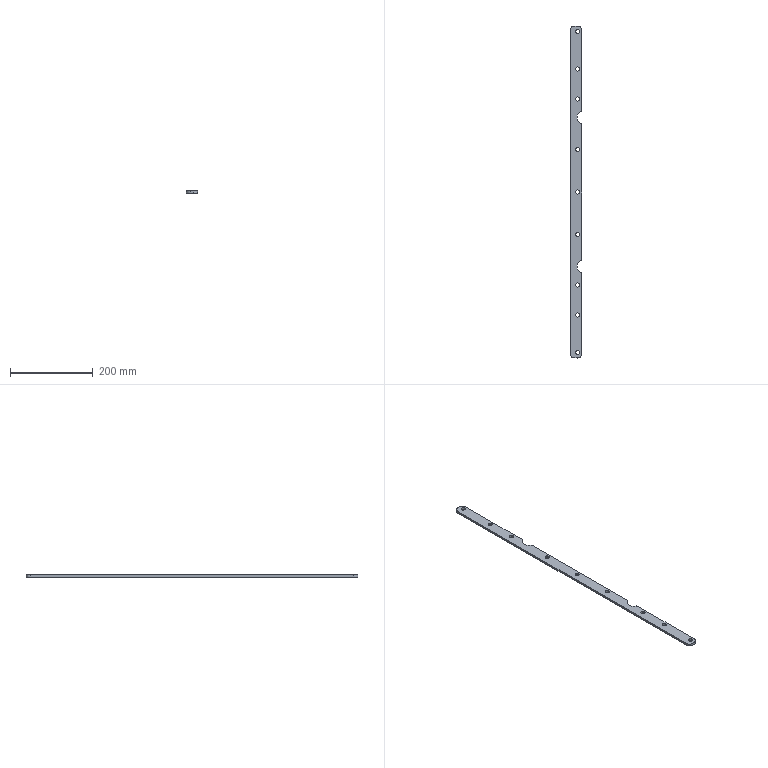Part | NX | features BREP 1 | 1 solid | 36 faces | box 27 x 803 x 5 mm | volume 101980 mm3 | cylinder 28 | plane 8 | commonest cylinder face diameters 10 x18 6 x4 20 x4 32 x2
STEP:
#1=CARTESIAN_POINT('',(541.715,-102.5,10.));
#2=VERTEX_POINT('',#1);
#3=CARTESIAN_POINT('',(551.715,-102.5,10.));
#4=VERTEX_POINT('',#3);
#5=CARTESIAN_POINT('',(546.715,-102.5,10.));
#6=DIRECTION('',(0.,0.,1.));
#7=DIRECTION('',(1.,0.,0.));
#8=AXIS2_PLACEMENT_3D('',#5,#6,#7);
#9=CIRCLE('',#8,5.);
#10=EDGE_CURVE('',#2,#4,#9,.T.);
#11=ORIENTED_EDGE('',*,*,#10,.F.);
#12=CARTESIAN_POINT('',(541.715,-102.5,15.));
#13=VERTEX_POINT('',#12);
#14=CARTESIAN_POINT('',(541.715,-102.5,20.));
#15=DIRECTION('',(0.,0.,1.));
#16=VECTOR('',#15,1000.);
#17=LINE('',#14,#16);
#18=EDGE_CURVE('',#2,#13,#17,.T.);
#19=ORIENTED_EDGE('',*,*,#18,.T.);
#20=CARTESIAN_POINT('',(551.715,-102.5,15.));
#21=VERTEX_POINT('',#20);
#22=CARTESIAN_POINT('',(546.715,-102.5,15.));
#23=DIRECTION('',(0.,0.,1.));
#24=DIRECTION('',(1.,0.,0.));
#25=AXIS2_PLACEMENT_3D('',#22,#23,#24);
#26=CIRCLE('',#25,5.);
#27=EDGE_CURVE('',#13,#21,#26,.T.);
#28=ORIENTED_EDGE('',*,*,#27,.T.);
#29=CARTESIAN_POINT('',(551.715,-102.5,20.));
#30=DIRECTION('',(0.,0.,1.));
#31=VECTOR('',#30,1000.);
#32=LINE('',#29,#31);
#33=EDGE_CURVE('',#4,#21,#32,.T.);
#34=ORIENTED_EDGE('',*,*,#33,.F.);
#35=EDGE_LOOP('',(#11,#19,#28,#34));
#36=FACE_BOUND('',#35,.T.);
#37=CARTESIAN_POINT('',(546.715,-102.5,20.));
#38=DIRECTION('',(0.,0.,1.));
#39=DIRECTION('',(-1.,0.,0.));
#40=AXIS2_PLACEMENT_3D('',#37,#38,#39);
#41=CYLINDRICAL_SURFACE('',#40,5.);
#42=ADVANCED_FACE('',(#36),#41,.F.);
#43=CARTESIAN_POINT('',(541.715,-0.0003019,10.));
#44=VERTEX_POINT('',#43);
#45=CARTESIAN_POINT('',(551.715,-0.0003019,10.));
#46=VERTEX_POINT('',#45);
#47=CARTESIAN_POINT('',(546.715,-0.0003019,10.));
#48=DIRECTION('',(0.,0.,1.));
#49=DIRECTION('',(1.,0.,0.));
#50=AXIS2_PLACEMENT_3D('',#47,#48,#49);
#51=CIRCLE('',#50,5.);
#52=EDGE_CURVE('',#44,#46,#51,.T.);
#53=ORIENTED_EDGE('',*,*,#52,.F.);
#54=CARTESIAN_POINT('',(541.715,-0.0003019,15.));
#55=VERTEX_POINT('',#54);
#56=CARTESIAN_POINT('',(541.715,-0.0003019,20.));
#57=DIRECTION('',(0.,0.,1.));
#58=VECTOR('',#57,1000.);
#59=LINE('',#56,#58);
#60=EDGE_CURVE('',#44,#55,#59,.T.);
#61=ORIENTED_EDGE('',*,*,#60,.T.);
#62=CARTESIAN_POINT('',(551.715,-0.0003019,15.));
#63=VERTEX_POINT('',#62);
#64=CARTESIAN_POINT('',(546.715,-0.0003019,15.));
#65=DIRECTION('',(0.,0.,1.));
#66=DIRECTION('',(1.,0.,0.));
#67=AXIS2_PLACEMENT_3D('',#64,#65,#66);
#68=CIRCLE('',#67,5.);
#69=EDGE_CURVE('',#55,#63,#68,.T.);
#70=ORIENTED_EDGE('',*,*,#69,.T.);
#71=CARTESIAN_POINT('',(551.715,-0.0003019,20.));
#72=DIRECTION('',(0.,0.,1.));
#73=VECTOR('',#72,1000.);
#74=LINE('',#71,#73);
#75=EDGE_CURVE('',#46,#63,#74,.T.);
#76=ORIENTED_EDGE('',*,*,#75,.F.);
#77=EDGE_LOOP('',(#53,#61,#70,#76));
#78=FACE_BOUND('',#77,.T.);
#79=CARTESIAN_POINT('',(546.715,-0.0003019,20.));
#80=DIRECTION('',(0.,0.,1.));
#81=DIRECTION('',(-1.,0.,0.));
#82=AXIS2_PLACEMENT_3D('',#79,#80,#81);
#83=CYLINDRICAL_SURFACE('',#82,5.);
#84=ADVANCED_FACE('',(#78),#83,.F.);
#85=CARTESIAN_POINT('',(541.715,102.5,10.));
#86=VERTEX_POINT('',#85);
#87=CARTESIAN_POINT('',(551.715,102.5,10.));
#88=VERTEX_POINT('',#87);
#89=CARTESIAN_POINT('',(546.715,102.5,10.));
#90=DIRECTION('',(0.,0.,1.));
#91=DIRECTION('',(1.,0.,0.));
#92=AXIS2_PLACEMENT_3D('',#89,#90,#91);
#93=CIRCLE('',#92,5.);
#94=EDGE_CURVE('',#86,#88,#93,.T.);
#95=ORIENTED_EDGE('',*,*,#94,.F.);
#96=CARTESIAN_POINT('',(541.715,102.5,15.));
#97=VERTEX_POINT('',#96);
#98=CARTESIAN_POINT('',(541.715,102.5,20.));
#99=DIRECTION('',(0.,0.,1.));
#100=VECTOR('',#99,1000.);
#101=LINE('',#98,#100);
#102=EDGE_CURVE('',#86,#97,#101,.T.);
#103=ORIENTED_EDGE('',*,*,#102,.T.);
#104=CARTESIAN_POINT('',(551.715,102.5,15.));
#105=VERTEX_POINT('',#104);
#106=CARTESIAN_POINT('',(546.715,102.5,15.));
#107=DIRECTION('',(0.,0.,1.));
#108=DIRECTION('',(1.,0.,0.));
#109=AXIS2_PLACEMENT_3D('',#106,#107,#108);
#110=CIRCLE('',#109,5.);
#111=EDGE_CURVE('',#97,#105,#110,.T.);
#112=ORIENTED_EDGE('',*,*,#111,.T.);
#113=CARTESIAN_POINT('',(551.715,102.5,20.));
#114=DIRECTION('',(0.,0.,1.));
#115=VECTOR('',#114,1000.);
#116=LINE('',#113,#115);
#117=EDGE_CURVE('',#88,#105,#116,.T.);
#118=ORIENTED_EDGE('',*,*,#117,.F.);
#119=EDGE_LOOP('',(#95,#103,#112,#118));
#120=FACE_BOUND('',#119,.T.);
#121=CARTESIAN_POINT('',(546.715,102.5,20.));
#122=DIRECTION('',(0.,0.,1.));
#123=DIRECTION('',(-1.,0.,0.));
#124=AXIS2_PLACEMENT_3D('',#121,#122,#123);
#125=CYLINDRICAL_SURFACE('',#124,5.);
#126=ADVANCED_FACE('',(#120),#125,.F.);
#127=CARTESIAN_POINT('',(541.715,225.,10.));
#128=VERTEX_POINT('',#127);
#129=CARTESIAN_POINT('',(551.715,225.,10.));
#130=VERTEX_POINT('',#129);
#131=CARTESIAN_POINT('',(546.715,225.,10.));
#132=DIRECTION('',(0.,0.,1.));
#133=DIRECTION('',(1.,0.,0.));
#134=AXIS2_PLACEMENT_3D('',#131,#132,#133);
#135=CIRCLE('',#134,5.);
#136=EDGE_CURVE('',#128,#130,#135,.T.);
#137=ORIENTED_EDGE('',*,*,#136,.F.);
#138=CARTESIAN_POINT('',(541.715,225.,15.));
#139=VERTEX_POINT('',#138);
#140=CARTESIAN_POINT('',(541.715,225.,20.));
#141=DIRECTION('',(0.,0.,1.));
#142=VECTOR('',#141,1000.);
#143=LINE('',#140,#142);
#144=EDGE_CURVE('',#128,#139,#143,.T.);
#145=ORIENTED_EDGE('',*,*,#144,.T.);
#146=CARTESIAN_POINT('',(551.715,225.,15.));
#147=VERTEX_POINT('',#146);
#148=CARTESIAN_POINT('',(546.715,225.,15.));
#149=DIRECTION('',(0.,0.,1.));
#150=DIRECTION('',(1.,0.,0.));
#151=AXIS2_PLACEMENT_3D('',#148,#149,#150);
#152=CIRCLE('',#151,5.);
#153=EDGE_CURVE('',#139,#147,#152,.T.);
#154=ORIENTED_EDGE('',*,*,#153,.T.);
#155=CARTESIAN_POINT('',(551.715,225.,20.));
#156=DIRECTION('',(0.,0.,1.));
#157=VECTOR('',#156,1000.);
#158=LINE('',#155,#157);
#159=EDGE_CURVE('',#130,#147,#158,.T.);
#160=ORIENTED_EDGE('',*,*,#159,.F.);
#161=EDGE_LOOP('',(#137,#145,#154,#160));
#162=FACE_BOUND('',#161,.T.);
#163=CARTESIAN_POINT('',(546.715,225.,20.));
#164=DIRECTION('',(0.,0.,1.));
#165=DIRECTION('',(-1.,0.,0.));
#166=AXIS2_PLACEMENT_3D('',#163,#164,#165);
#167=CYLINDRICAL_SURFACE('',#166,5.);
#168=ADVANCED_FACE('',(#162),#167,.F.);
#169=CARTESIAN_POINT('',(541.715,297.5,10.));
#170=VERTEX_POINT('',#169);
#171=CARTESIAN_POINT('',(551.715,297.5,10.));
#172=VERTEX_POINT('',#171);
#173=CARTESIAN_POINT('',(546.715,297.5,10.));
#174=DIRECTION('',(0.,0.,1.));
#175=DIRECTION('',(1.,0.,0.));
#176=AXIS2_PLACEMENT_3D('',#173,#174,#175);
#177=CIRCLE('',#176,5.);
#178=EDGE_CURVE('',#170,#172,#177,.T.);
#179=ORIENTED_EDGE('',*,*,#178,.F.);
#180=CARTESIAN_POINT('',(541.715,297.5,15.));
#181=VERTEX_POINT('',#180);
#182=CARTESIAN_POINT('',(541.715,297.5,20.));
#183=DIRECTION('',(0.,0.,1.));
#184=VECTOR('',#183,1000.);
#185=LINE('',#182,#184);
#186=EDGE_CURVE('',#170,#181,#185,.T.);
#187=ORIENTED_EDGE('',*,*,#186,.T.);
#188=CARTESIAN_POINT('',(551.715,297.5,15.));
#189=VERTEX_POINT('',#188);
#190=CARTESIAN_POINT('',(546.715,297.5,15.));
#191=DIRECTION('',(0.,0.,1.));
#192=DIRECTION('',(1.,0.,0.));
#193=AXIS2_PLACEMENT_3D('',#190,#191,#192);
#194=CIRCLE('',#193,5.);
#195=EDGE_CURVE('',#181,#189,#194,.T.);
#196=ORIENTED_EDGE('',*,*,#195,.T.);
#197=CARTESIAN_POINT('',(551.715,297.5,20.));
#198=DIRECTION('',(0.,0.,1.));
#199=VECTOR('',#198,1000.);
#200=LINE('',#197,#199);
#201=EDGE_CURVE('',#172,#189,#200,.T.);
#202=ORIENTED_EDGE('',*,*,#201,.F.);
#203=EDGE_LOOP('',(#179,#187,#196,#202));
#204=FACE_BOUND('',#203,.T.);
#205=CARTESIAN_POINT('',(546.715,297.5,20.));
#206=DIRECTION('',(0.,0.,1.));
#207=DIRECTION('',(-1.,0.,0.));
#208=AXIS2_PLACEMENT_3D('',#205,#206,#207);
#209=CYLINDRICAL_SURFACE('',#208,5.);
#210=ADVANCED_FACE('',(#204),#209,.F.);
#211=CARTESIAN_POINT('',(541.715,-297.5,10.));
#212=VERTEX_POINT('',#211);
#213=CARTESIAN_POINT('',(551.715,-297.5,10.));
#214=VERTEX_POINT('',#213);
#215=CARTESIAN_POINT('',(546.715,-297.5,10.));
#216=DIRECTION('',(0.,0.,1.));
#217=DIRECTION('',(1.,0.,0.));
#218=AXIS2_PLACEMENT_3D('',#215,#216,#217);
#219=CIRCLE('',#218,5.);
#220=EDGE_CURVE('',#212,#214,#219,.T.);
#221=ORIENTED_EDGE('',*,*,#220,.F.);
#222=CARTESIAN_POINT('',(541.715,-297.5,15.));
#223=VERTEX_POINT('',#222);
#224=CARTESIAN_POINT('',(541.715,-297.5,20.));
#225=DIRECTION('',(0.,0.,1.));
#226=VECTOR('',#225,1000.);
#227=LINE('',#224,#226);
#228=EDGE_CURVE('',#212,#223,#227,.T.);
#229=ORIENTED_EDGE('',*,*,#228,.T.);
#230=CARTESIAN_POINT('',(551.715,-297.5,15.));
#231=VERTEX_POINT('',#230);
#232=CARTESIAN_POINT('',(546.715,-297.5,15.));
#233=DIRECTION('',(0.,0.,1.));
#234=DIRECTION('',(1.,0.,0.));
#235=AXIS2_PLACEMENT_3D('',#232,#233,#234);
#236=CIRCLE('',#235,5.);
#237=EDGE_CURVE('',#223,#231,#236,.T.);
#238=ORIENTED_EDGE('',*,*,#237,.T.);
#239=CARTESIAN_POINT('',(551.715,-297.5,20.));
#240=DIRECTION('',(0.,0.,1.));
#241=VECTOR('',#240,1000.);
#242=LINE('',#239,#241);
#243=EDGE_CURVE('',#214,#231,#242,.T.);
#244=ORIENTED_EDGE('',*,*,#243,.F.);
#245=EDGE_LOOP('',(#221,#229,#238,#244));
#246=FACE_BOUND('',#245,.T.);
#247=CARTESIAN_POINT('',(546.715,-297.5,20.));
#248=DIRECTION('',(0.,0.,1.));
#249=DIRECTION('',(-1.,0.,0.));
#250=AXIS2_PLACEMENT_3D('',#247,#248,#249);
#251=CYLINDRICAL_SURFACE('',#250,5.);
#252=ADVANCED_FACE('',(#246),#251,.F.);
#253=CARTESIAN_POINT('',(541.715,-388.5,10.));
#254=VERTEX_POINT('',#253);
#255=CARTESIAN_POINT('',(551.715,-388.5,10.));
#256=VERTEX_POINT('',#255);
#257=CARTESIAN_POINT('',(546.715,-388.5,10.));
#258=DIRECTION('',(0.,0.,1.));
#259=DIRECTION('',(1.,0.,0.));
#260=AXIS2_PLACEMENT_3D('',#257,#258,#259);
#261=CIRCLE('',#260,5.);
#262=EDGE_CURVE('',#254,#256,#261,.T.);
#263=ORIENTED_EDGE('',*,*,#262,.F.);
#264=CARTESIAN_POINT('',(541.715,-388.5,15.));
#265=VERTEX_POINT('',#264);
#266=CARTESIAN_POINT('',(541.715,-388.5,15.));
#267=DIRECTION('',(0.,0.,1.));
#268=VECTOR('',#267,1000.);
#269=LINE('',#266,#268);
#270=EDGE_CURVE('',#254,#265,#269,.T.);
#271=ORIENTED_EDGE('',*,*,#270,.T.);
#272=CARTESIAN_POINT('',(551.715,-388.5,15.));
#273=VERTEX_POINT('',#272);
#274=CARTESIAN_POINT('',(546.715,-388.5,15.));
#275=DIRECTION('',(0.,0.,1.));
#276=DIRECTION('',(1.,0.,0.));
#277=AXIS2_PLACEMENT_3D('',#274,#275,#276);
#278=CIRCLE('',#277,5.);
#279=EDGE_CURVE('',#265,#273,#278,.T.);
#280=ORIENTED_EDGE('',*,*,#279,.T.);
#281=CARTESIAN_POINT('',(551.715,-388.5,15.));
#282=DIRECTION('',(0.,0.,1.));
#283=VECTOR('',#282,1000.);
#284=LINE('',#281,#283);
#285=EDGE_CURVE('',#256,#273,#284,.T.);
#286=ORIENTED_EDGE('',*,*,#285,.F.);
#287=EDGE_LOOP('',(#263,#271,#280,#286));
#288=FACE_BOUND('',#287,.T.);
#289=CARTESIAN_POINT('',(546.715,-388.5,15.));
#290=DIRECTION('',(0.,0.,1.));
#291=DIRECTION('',(-1.,0.,0.));
#292=AXIS2_PLACEMENT_3D('',#289,#290,#291);
#293=CYLINDRICAL_SURFACE('',#292,5.);
#294=ADVANCED_FACE('',(#288),#293,.F.);
#295=CARTESIAN_POINT('',(541.715,388.5,10.));
#296=VERTEX_POINT('',#295);
#297=CARTESIAN_POINT('',(551.715,388.5,10.));
#298=VERTEX_POINT('',#297);
#299=CARTESIAN_POINT('',(546.715,388.5,10.));
#300=DIRECTION('',(0.,0.,1.));
#301=DIRECTION('',(1.,0.,0.));
#302=AXIS2_PLACEMENT_3D('',#299,#300,#301);
#303=CIRCLE('',#302,5.);
#304=EDGE_CURVE('',#296,#298,#303,.T.);
#305=ORIENTED_EDGE('',*,*,#304,.F.);
#306=CARTESIAN_POINT('',(541.715,388.5,15.));
#307=VERTEX_POINT('',#306);
#308=CARTESIAN_POINT('',(541.715,388.5,15.));
#309=DIRECTION('',(0.,0.,1.));
#310=VECTOR('',#309,1000.);
#311=LINE('',#308,#310);
#312=EDGE_CURVE('',#296,#307,#311,.T.);
#313=ORIENTED_EDGE('',*,*,#312,.T.);
#314=CARTESIAN_POINT('',(551.715,388.5,15.));
#315=VERTEX_POINT('',#314);
#316=CARTESIAN_POINT('',(546.715,388.5,15.));
#317=DIRECTION('',(0.,0.,1.));
#318=DIRECTION('',(1.,0.,0.));
#319=AXIS2_PLACEMENT_3D('',#316,#317,#318);
#320=CIRCLE('',#319,5.);
#321=EDGE_CURVE('',#307,#315,#320,.T.);
#322=ORIENTED_EDGE('',*,*,#321,.T.);
#323=CARTESIAN_POINT('',(551.715,388.5,15.));
#324=DIRECTION('',(0.,0.,1.));
#325=VECTOR('',#324,1000.);
#326=LINE('',#323,#325);
#327=EDGE_CURVE('',#298,#315,#326,.T.);
#328=ORIENTED_EDGE('',*,*,#327,.F.);
#329=EDGE_LOOP('',(#305,#313,#322,#328));
#330=FACE_BOUND('',#329,.T.);
#331=CARTESIAN_POINT('',(546.715,388.5,15.));
#332=DIRECTION('',(0.,0.,1.));
#333=DIRECTION('',(-1.,0.,0.));
#334=AXIS2_PLACEMENT_3D('',#331,#332,#333);
#335=CYLINDRICAL_SURFACE('',#334,5.);
#336=ADVANCED_FACE('',(#330),#335,.F.);
#337=CARTESIAN_POINT('',(541.715,-225.,10.));
#338=VERTEX_POINT('',#337);
#339=CARTESIAN_POINT('',(551.715,-225.,10.));
#340=VERTEX_POINT('',#339);
#341=CARTESIAN_POINT('',(546.715,-225.,10.));
#342=DIRECTION('',(0.,0.,1.));
#343=DIRECTION('',(1.,0.,0.));
#344=AXIS2_PLACEMENT_3D('',#341,#342,#343);
#345=CIRCLE('',#344,5.);
#346=EDGE_CURVE('',#338,#340,#345,.T.);
#347=ORIENTED_EDGE('',*,*,#346,.F.);
#348=CARTESIAN_POINT('',(541.715,-225.,15.));
#349=VERTEX_POINT('',#348);
#350=CARTESIAN_POINT('',(541.715,-225.,20.));
#351=DIRECTION('',(0.,0.,1.));
#352=VECTOR('',#351,1000.);
#353=LINE('',#350,#352);
#354=EDGE_CURVE('',#338,#349,#353,.T.);
#355=ORIENTED_EDGE('',*,*,#354,.T.);
#356=CARTESIAN_POINT('',(551.715,-225.,15.));
#357=VERTEX_POINT('',#356);
#358=CARTESIAN_POINT('',(546.715,-225.,15.));
#359=DIRECTION('',(0.,0.,1.));
#360=DIRECTION('',(1.,0.,0.));
#361=AXIS2_PLACEMENT_3D('',#358,#359,#360);
#362=CIRCLE('',#361,5.);
#363=EDGE_CURVE('',#349,#357,#362,.T.);
#364=ORIENTED_EDGE('',*,*,#363,.T.);
#365=CARTESIAN_POINT('',(551.715,-225.,20.));
#366=DIRECTION('',(0.,0.,1.));
#367=VECTOR('',#366,1000.);
#368=LINE('',#365,#367);
#369=EDGE_CURVE('',#340,#357,#368,.T.);
#370=ORIENTED_EDGE('',*,*,#369,.F.);
#371=EDGE_LOOP('',(#347,#355,#364,#370));
#372=FACE_BOUND('',#371,.T.);
#373=CARTESIAN_POINT('',(546.715,-225.,20.));
#374=DIRECTION('',(0.,0.,1.));
#375=DIRECTION('',(-1.,0.,0.));
#376=AXIS2_PLACEMENT_3D('',#373,#374,#375);
#377=CYLINDRICAL_SURFACE('',#376,5.);
#378=ADVANCED_FACE('',(#372),#377,.F.);
#379=CARTESIAN_POINT('',(556.16,-197.334,15.));
#380=VERTEX_POINT('',#379);
#381=CARTESIAN_POINT('',(556.16,-391.5,15.));
#382=VERTEX_POINT('',#381);
#383=CARTESIAN_POINT('',(556.16,-0.0003019,15.));
#384=DIRECTION('',(0.,-1.,0.));
#385=VECTOR('',#384,1000.);
#386=LINE('',#383,#385);
#387=EDGE_CURVE('',#380,#382,#386,.T.);
#388=ORIENTED_EDGE('',*,*,#387,.F.);
#389=CARTESIAN_POINT('',(554.423,-194.613,15.));
#390=VERTEX_POINT('',#389);
#391=CARTESIAN_POINT('',(553.16,-197.334,15.));
#392=DIRECTION('',(0.,0.,-1.));
#393=DIRECTION('',(-1.,0.,0.));
#394=AXIS2_PLACEMENT_3D('',#391,#392,#393);
#395=CIRCLE('',#394,3.);
#396=EDGE_CURVE('',#390,#380,#395,.T.);
#397=ORIENTED_EDGE('',*,*,#396,.F.);
#398=CARTESIAN_POINT('',(554.423,-165.587,15.));
#399=VERTEX_POINT('',#398);
#400=CARTESIAN_POINT('',(561.16,-180.1,15.));
#401=DIRECTION('',(0.,0.,1.));
#402=DIRECTION('',(1.,0.,0.));
#403=AXIS2_PLACEMENT_3D('',#400,#401,#402);
#404=CIRCLE('',#403,16.);
#405=EDGE_CURVE('',#399,#390,#404,.T.);
#406=ORIENTED_EDGE('',*,*,#405,.F.);
#407=CARTESIAN_POINT('',(556.16,-162.866,15.));
#408=VERTEX_POINT('',#407);
#409=CARTESIAN_POINT('',(553.16,-162.866,15.));
#410=DIRECTION('',(0.,0.,-1.));
#411=DIRECTION('',(1.,0.,0.));
#412=AXIS2_PLACEMENT_3D('',#409,#410,#411);
#413=CIRCLE('',#412,3.);
#414=EDGE_CURVE('',#408,#399,#413,.T.);
#415=ORIENTED_EDGE('',*,*,#414,.F.);
#416=CARTESIAN_POINT('',(556.16,162.866,15.));
#417=VERTEX_POINT('',#416);
#418=CARTESIAN_POINT('',(556.16,-0.0003019,15.));
#419=DIRECTION('',(0.,-1.,0.));
#420=VECTOR('',#419,1000.);
#421=LINE('',#418,#420);
#422=EDGE_CURVE('',#417,#408,#421,.T.);
#423=ORIENTED_EDGE('',*,*,#422,.F.);
#424=CARTESIAN_POINT('',(554.423,165.587,15.));
#425=VERTEX_POINT('',#424);
#426=CARTESIAN_POINT('',(553.16,162.866,15.));
#427=DIRECTION('',(0.,0.,-1.));
#428=DIRECTION('',(-1.,0.,0.));
#429=AXIS2_PLACEMENT_3D('',#426,#427,#428);
#430=CIRCLE('',#429,3.);
#431=EDGE_CURVE('',#425,#417,#430,.T.);
#432=ORIENTED_EDGE('',*,*,#431,.F.);
#433=CARTESIAN_POINT('',(554.423,194.613,15.));
#434=VERTEX_POINT('',#433);
#435=CARTESIAN_POINT('',(561.16,180.1,15.));
#436=DIRECTION('',(0.,0.,1.));
#437=DIRECTION('',(1.,0.,0.));
#438=AXIS2_PLACEMENT_3D('',#435,#436,#437);
#439=CIRCLE('',#438,16.);
#440=EDGE_CURVE('',#434,#425,#439,.T.);
#441=ORIENTED_EDGE('',*,*,#440,.F.);
#442=CARTESIAN_POINT('',(556.16,197.334,15.));
#443=VERTEX_POINT('',#442);
#444=CARTESIAN_POINT('',(553.16,197.334,15.));
#445=DIRECTION('',(0.,0.,-1.));
#446=DIRECTION('',(1.,0.,0.));
#447=AXIS2_PLACEMENT_3D('',#444,#445,#446);
#448=CIRCLE('',#447,3.);
#449=EDGE_CURVE('',#443,#434,#448,.T.);
#450=ORIENTED_EDGE('',*,*,#449,.F.);
#451=CARTESIAN_POINT('',(556.16,391.5,15.));
#452=VERTEX_POINT('',#451);
#453=CARTESIAN_POINT('',(556.16,-0.0003019,15.));
#454=DIRECTION('',(0.,-1.,0.));
#455=VECTOR('',#454,1000.);
#456=LINE('',#453,#455);
#457=EDGE_CURVE('',#452,#443,#456,.T.);
#458=ORIENTED_EDGE('',*,*,#457,.F.);
#459=CARTESIAN_POINT('',(546.16,401.5,15.));
#460=VERTEX_POINT('',#459);
#461=CARTESIAN_POINT('',(546.16,391.5,15.));
#462=DIRECTION('',(0.,0.,-1.));
#463=DIRECTION('',(1.,0.,0.));
#464=AXIS2_PLACEMENT_3D('',#461,#462,#463);
#465=CIRCLE('',#464,10.);
#466=EDGE_CURVE('',#460,#452,#465,.T.);
#467=ORIENTED_EDGE('',*,*,#466,.F.);
#468=CARTESIAN_POINT('',(539.16,401.5,15.));
#469=VERTEX_POINT('',#468);
#470=CARTESIAN_POINT('',(-11.34,401.5,15.));
#471=DIRECTION('',(1.,0.,0.));
#472=VECTOR('',#471,1000.);
#473=LINE('',#470,#472);
#474=EDGE_CURVE('',#469,#460,#473,.T.);
#475=ORIENTED_EDGE('',*,*,#474,.F.);
#476=CARTESIAN_POINT('',(529.16,391.5,15.));
#477=VERTEX_POINT('',#476);
#478=CARTESIAN_POINT('',(539.16,391.5,15.));
#479=DIRECTION('',(0.,0.,-1.));
#480=DIRECTION('',(-1.,0.,0.));
#481=AXIS2_PLACEMENT_3D('',#478,#479,#480);
#482=CIRCLE('',#481,10.);
#483=EDGE_CURVE('',#477,#469,#482,.T.);
#484=ORIENTED_EDGE('',*,*,#483,.F.);
#485=CARTESIAN_POINT('',(529.16,-391.5,15.));
#486=VERTEX_POINT('',#485);
#487=CARTESIAN_POINT('',(529.16,-0.0003019,15.));
#488=DIRECTION('',(0.,1.,0.));
#489=VECTOR('',#488,1000.);
#490=LINE('',#487,#489);
#491=EDGE_CURVE('',#486,#477,#490,.T.);
#492=ORIENTED_EDGE('',*,*,#491,.F.);
#493=CARTESIAN_POINT('',(539.16,-401.5,15.));
#494=VERTEX_POINT('',#493);
#495=CARTESIAN_POINT('',(539.16,-391.5,15.));
#496=DIRECTION('',(0.,0.,-1.));
#497=DIRECTION('',(-1.,0.,0.));
#498=AXIS2_PLACEMENT_3D('',#495,#496,#497);
#499=CIRCLE('',#498,10.);
#500=EDGE_CURVE('',#494,#486,#499,.T.);
#501=ORIENTED_EDGE('',*,*,#500,.F.);
#502=CARTESIAN_POINT('',(546.16,-401.5,15.));
#503=VERTEX_POINT('',#502);
#504=CARTESIAN_POINT('',(-11.34,-401.5,15.));
#505=DIRECTION('',(-1.,0.,0.));
#506=VECTOR('',#505,1000.);
#507=LINE('',#504,#506);
#508=EDGE_CURVE('',#503,#494,#507,.T.);
#509=ORIENTED_EDGE('',*,*,#508,.F.);
#510=CARTESIAN_POINT('',(546.16,-391.5,15.));
#511=DIRECTION('',(0.,0.,-1.));
#512=DIRECTION('',(1.,0.,0.));
#513=AXIS2_PLACEMENT_3D('',#510,#511,#512);
#514=CIRCLE('',#513,10.);
#515=EDGE_CURVE('',#382,#503,#514,.T.);
#516=ORIENTED_EDGE('',*,*,#515,.F.);
#517=EDGE_LOOP('',(#388,#397,#406,#415,#423,#432,#441,#450,#458,#467,#475,#484,#492,#501,#509,#516));
#518=FACE_BOUND('',#517,.T.);
#519=CARTESIAN_POINT('',(546.715,-102.5,15.));
#520=DIRECTION('',(0.,0.,1.));
#521=DIRECTION('',(1.,0.,0.));
#522=AXIS2_PLACEMENT_3D('',#519,#520,#521);
#523=CIRCLE('',#522,5.);
#524=EDGE_CURVE('',#21,#13,#523,.T.);
#525=ORIENTED_EDGE('',*,*,#524,.F.);
#526=ORIENTED_EDGE('',*,*,#27,.F.);
#527=EDGE_LOOP('',(#525,#526));
#528=FACE_BOUND('',#527,.T.);
#529=CARTESIAN_POINT('',(546.715,-0.0003019,15.));
#530=DIRECTION('',(0.,0.,1.));
#531=DIRECTION('',(1.,0.,0.));
#532=AXIS2_PLACEMENT_3D('',#529,#530,#531);
#533=CIRCLE('',#532,5.);
#534=EDGE_CURVE('',#63,#55,#533,.T.);
#535=ORIENTED_EDGE('',*,*,#534,.F.);
#536=ORIENTED_EDGE('',*,*,#69,.F.);
#537=EDGE_LOOP('',(#535,#536));
#538=FACE_BOUND('',#537,.T.);
#539=CARTESIAN_POINT('',(546.715,102.5,15.));
#540=DIRECTION('',(0.,0.,1.));
#541=DIRECTION('',(1.,0.,0.));
#542=AXIS2_PLACEMENT_3D('',#539,#540,#541);
#543=CIRCLE('',#542,5.);
#544=EDGE_CURVE('',#105,#97,#543,.T.);
#545=ORIENTED_EDGE('',*,*,#544,.F.);
#546=ORIENTED_EDGE('',*,*,#111,.F.);
#547=EDGE_LOOP('',(#545,#546));
#548=FACE_BOUND('',#547,.T.);
#549=CARTESIAN_POINT('',(546.715,225.,15.));
#550=DIRECTION('',(0.,0.,1.));
#551=DIRECTION('',(1.,0.,0.));
#552=AXIS2_PLACEMENT_3D('',#549,#550,#551);
#553=CIRCLE('',#552,5.);
#554=EDGE_CURVE('',#147,#139,#553,.T.);
#555=ORIENTED_EDGE('',*,*,#554,.F.);
#556=ORIENTED_EDGE('',*,*,#153,.F.);
#557=EDGE_LOOP('',(#555,#556));
#558=FACE_BOUND('',#557,.T.);
#559=CARTESIAN_POINT('',(546.715,297.5,15.));
#560=DIRECTION('',(0.,0.,1.));
#561=DIRECTION('',(1.,0.,0.));
#562=AXIS2_PLACEMENT_3D('',#559,#560,#561);
#563=CIRCLE('',#562,5.);
#564=EDGE_CURVE('',#189,#181,#563,.T.);
#565=ORIENTED_EDGE('',*,*,#564,.F.);
#566=ORIENTED_EDGE('',*,*,#195,.F.);
#567=EDGE_LOOP('',(#565,#566));
#568=FACE_BOUND('',#567,.T.);
#569=CARTESIAN_POINT('',(546.715,-297.5,15.));
#570=DIRECTION('',(0.,0.,1.));
#571=DIRECTION('',(1.,0.,0.));
#572=AXIS2_PLACEMENT_3D('',#569,#570,#571);
#573=CIRCLE('',#572,5.);
#574=EDGE_CURVE('',#231,#223,#573,.T.);
#575=ORIENTED_EDGE('',*,*,#574,.F.);
#576=ORIENTED_EDGE('',*,*,#237,.F.);
#577=EDGE_LOOP('',(#575,#576));
#578=FACE_BOUND('',#577,.T.);
#579=CARTESIAN_POINT('',(546.715,-388.5,15.));
#580=DIRECTION('',(0.,0.,1.));
#581=DIRECTION('',(1.,0.,0.));
#582=AXIS2_PLACEMENT_3D('',#579,#580,#581);
#583=CIRCLE('',#582,5.);
#584=EDGE_CURVE('',#273,#265,#583,.T.);
#585=ORIENTED_EDGE('',*,*,#584,.F.);
#586=ORIENTED_EDGE('',*,*,#279,.F.);
#587=EDGE_LOOP('',(#585,#586));
#588=FACE_BOUND('',#587,.T.);
#589=CARTESIAN_POINT('',(546.715,388.5,15.));
#590=DIRECTION('',(0.,0.,1.));
#591=DIRECTION('',(1.,0.,0.));
#592=AXIS2_PLACEMENT_3D('',#589,#590,#591);
#593=CIRCLE('',#592,5.);
#594=EDGE_CURVE('',#315,#307,#593,.T.);
#595=ORIENTED_EDGE('',*,*,#594,.F.);
#596=ORIENTED_EDGE('',*,*,#321,.F.);
#597=EDGE_LOOP('',(#595,#596));
#598=FACE_BOUND('',#597,.T.);
#599=CARTESIAN_POINT('',(546.715,-225.,15.));
#600=DIRECTION('',(0.,0.,1.));
#601=DIRECTION('',(1.,0.,0.));
#602=AXIS2_PLACEMENT_3D('',#599,#600,#601);
#603=CIRCLE('',#602,5.);
#604=EDGE_CURVE('',#357,#349,#603,.T.);
#605=ORIENTED_EDGE('',*,*,#604,.F.);
#606=ORIENTED_EDGE('',*,*,#363,.F.);
#607=EDGE_LOOP('',(#605,#606));
#608=FACE_BOUND('',#607,.T.);
#609=CARTESIAN_POINT('',(-11.34,-0.0003019,15.));
#610=DIRECTION('',(0.,0.,-1.));
#611=DIRECTION('',(1.,0.,0.));
#612=AXIS2_PLACEMENT_3D('',#609,#610,#611);
#613=PLANE('',#612);
#614=ADVANCED_FACE('',(#518,#528,#538,#548,#558,#568,#578,#588,#598,#608),#613,.F.);
#615=CARTESIAN_POINT('',(556.16,-391.5,10.));
#616=VERTEX_POINT('',#615);
#617=CARTESIAN_POINT('',(556.16,-391.5,-2.53));
#618=DIRECTION('',(0.,0.,1.));
#619=VECTOR('',#618,1000.);
#620=LINE('',#617,#619);
#621=EDGE_CURVE('',#616,#382,#620,.T.);
#622=ORIENTED_EDGE('',*,*,#621,.T.);
#623=ORIENTED_EDGE('',*,*,#515,.T.);
#624=CARTESIAN_POINT('',(546.16,-401.5,10.));
#625=VERTEX_POINT('',#624);
#626=CARTESIAN_POINT('',(546.16,-401.5,-2.53));
#627=DIRECTION('',(0.,0.,-1.));
#628=VECTOR('',#627,1000.);
#629=LINE('',#626,#628);
#630=EDGE_CURVE('',#503,#625,#629,.T.);
#631=ORIENTED_EDGE('',*,*,#630,.T.);
#632=CARTESIAN_POINT('',(546.16,-391.5,10.));
#633=DIRECTION('',(0.,0.,1.));
#634=DIRECTION('',(1.,0.,0.));
#635=AXIS2_PLACEMENT_3D('',#632,#633,#634);
#636=CIRCLE('',#635,10.);
#637=EDGE_CURVE('',#625,#616,#636,.T.);
#638=ORIENTED_EDGE('',*,*,#637,.T.);
#639=EDGE_LOOP('',(#622,#623,#631,#638));
#640=FACE_BOUND('',#639,.T.);
#641=CARTESIAN_POINT('',(546.16,-391.5,-2.53));
#642=DIRECTION('',(0.,0.,1.));
#643=DIRECTION('',(-1.,0.,0.));
#644=AXIS2_PLACEMENT_3D('',#641,#642,#643);
#645=CYLINDRICAL_SURFACE('',#644,10.);
#646=ADVANCED_FACE('',(#640),#645,.T.);
#647=ORIENTED_EDGE('',*,*,#387,.T.);
#648=ORIENTED_EDGE('',*,*,#621,.F.);
#649=CARTESIAN_POINT('',(556.16,-197.334,10.));
#650=VERTEX_POINT('',#649);
#651=CARTESIAN_POINT('',(556.16,390.,10.));
#652=DIRECTION('',(0.,1.,0.));
#653=VECTOR('',#652,1000.);
#654=LINE('',#651,#653);
#655=EDGE_CURVE('',#616,#650,#654,.T.);
#656=ORIENTED_EDGE('',*,*,#655,.T.);
#657=CARTESIAN_POINT('',(556.16,-197.334,15.));
#658=DIRECTION('',(0.,0.,1.));
#659=VECTOR('',#658,1000.);
#660=LINE('',#657,#659);
#661=EDGE_CURVE('',#650,#380,#660,.T.);
#662=ORIENTED_EDGE('',*,*,#661,.T.);
#663=EDGE_LOOP('',(#647,#648,#656,#662));
#664=FACE_BOUND('',#663,.T.);
#665=CARTESIAN_POINT('',(556.16,390.,15.));
#666=DIRECTION('',(1.,0.,0.));
#667=DIRECTION('',(0.,0.,1.));
#668=AXIS2_PLACEMENT_3D('',#665,#666,#667);
#669=PLANE('',#668);
#670=ADVANCED_FACE('',(#664),#669,.T.);
#671=CARTESIAN_POINT('',(554.423,-194.613,10.));
#672=VERTEX_POINT('',#671);
#673=CARTESIAN_POINT('',(554.423,-194.613,21.518));
#674=DIRECTION('',(0.,0.,1.));
#675=VECTOR('',#674,1000.);
#676=LINE('',#673,#675);
#677=EDGE_CURVE('',#672,#390,#676,.T.);
#678=ORIENTED_EDGE('',*,*,#677,.T.);
#679=ORIENTED_EDGE('',*,*,#396,.T.);
#680=ORIENTED_EDGE('',*,*,#661,.F.);
#681=CARTESIAN_POINT('',(553.16,-197.334,10.));
#682=DIRECTION('',(0.,0.,1.));
#683=DIRECTION('',(-1.,0.,0.));
#684=AXIS2_PLACEMENT_3D('',#681,#682,#683);
#685=CIRCLE('',#684,3.);
#686=EDGE_CURVE('',#650,#672,#685,.T.);
#687=ORIENTED_EDGE('',*,*,#686,.T.);
#688=EDGE_LOOP('',(#678,#679,#680,#687));
#689=FACE_BOUND('',#688,.T.);
#690=CARTESIAN_POINT('',(553.16,-197.334,21.518));
#691=DIRECTION('',(0.,0.,-1.));
#692=DIRECTION('',(1.,0.,0.));
#693=AXIS2_PLACEMENT_3D('',#690,#691,#692);
#694=CYLINDRICAL_SURFACE('',#693,3.);
#695=ADVANCED_FACE('',(#689),#694,.T.);
#696=ORIENTED_EDGE('',*,*,#405,.T.);
#697=ORIENTED_EDGE('',*,*,#677,.F.);
#698=CARTESIAN_POINT('',(554.423,-165.587,10.));
#699=VERTEX_POINT('',#698);
#700=CARTESIAN_POINT('',(561.16,-180.1,10.));
#701=DIRECTION('',(0.,0.,1.));
#702=DIRECTION('',(1.,0.,0.));
#703=AXIS2_PLACEMENT_3D('',#700,#701,#702);
#704=CIRCLE('',#703,16.);
#705=EDGE_CURVE('',#699,#672,#704,.T.);
#706=ORIENTED_EDGE('',*,*,#705,.F.);
#707=CARTESIAN_POINT('',(554.423,-165.587,-26.5));
#708=DIRECTION('',(0.,0.,-1.));
#709=VECTOR('',#708,1000.);
#710=LINE('',#707,#709);
#711=EDGE_CURVE('',#399,#699,#710,.T.);
#712=ORIENTED_EDGE('',*,*,#711,.F.);
#713=EDGE_LOOP('',(#696,#697,#706,#712));
#714=FACE_BOUND('',#713,.T.);
#715=CARTESIAN_POINT('',(561.16,-180.1,-26.5));
#716=DIRECTION('',(0.,0.,1.));
#717=DIRECTION('',(-1.,0.,0.));
#718=AXIS2_PLACEMENT_3D('',#715,#716,#717);
#719=CYLINDRICAL_SURFACE('',#718,16.);
#720=ADVANCED_FACE('',(#714),#719,.F.);
#721=ORIENTED_EDGE('',*,*,#711,.T.);
#722=CARTESIAN_POINT('',(556.16,-162.866,10.));
#723=VERTEX_POINT('',#722);
#724=CARTESIAN_POINT('',(553.16,-162.866,10.));
#725=DIRECTION('',(0.,0.,1.));
#726=DIRECTION('',(1.,0.,0.));
#727=AXIS2_PLACEMENT_3D('',#724,#725,#726);
#728=CIRCLE('',#727,3.);
#729=EDGE_CURVE('',#699,#723,#728,.T.);
#730=ORIENTED_EDGE('',*,*,#729,.T.);
#731=CARTESIAN_POINT('',(556.16,-162.866,3.482));
#732=DIRECTION('',(0.,0.,1.));
#733=VECTOR('',#732,1000.);
#734=LINE('',#731,#733);
#735=EDGE_CURVE('',#723,#408,#734,.T.);
#736=ORIENTED_EDGE('',*,*,#735,.T.);
#737=ORIENTED_EDGE('',*,*,#414,.T.);
#738=EDGE_LOOP('',(#721,#730,#736,#737));
#739=FACE_BOUND('',#738,.T.);
#740=CARTESIAN_POINT('',(553.16,-162.866,3.482));
#741=DIRECTION('',(0.,0.,1.));
#742=DIRECTION('',(-1.,0.,0.));
#743=AXIS2_PLACEMENT_3D('',#740,#741,#742);
#744=CYLINDRICAL_SURFACE('',#743,3.);
#745=ADVANCED_FACE('',(#739),#744,.T.);
#746=ORIENTED_EDGE('',*,*,#422,.T.);
#747=ORIENTED_EDGE('',*,*,#735,.F.);
#748=CARTESIAN_POINT('',(556.16,162.866,10.));
#749=VERTEX_POINT('',#748);
#750=CARTESIAN_POINT('',(556.16,390.,10.));
#751=DIRECTION('',(0.,1.,0.));
#752=VECTOR('',#751,1000.);
#753=LINE('',#750,#752);
#754=EDGE_CURVE('',#723,#749,#753,.T.);
#755=ORIENTED_EDGE('',*,*,#754,.T.);
#756=CARTESIAN_POINT('',(556.16,162.866,15.));
#757=DIRECTION('',(0.,0.,1.));
#758=VECTOR('',#757,1000.);
#759=LINE('',#756,#758);
#760=EDGE_CURVE('',#749,#417,#759,.T.);
#761=ORIENTED_EDGE('',*,*,#760,.T.);
#762=EDGE_LOOP('',(#746,#747,#755,#761));
#763=FACE_BOUND('',#762,.T.);
#764=CARTESIAN_POINT('',(556.16,390.,15.));
#765=DIRECTION('',(1.,0.,0.));
#766=DIRECTION('',(0.,0.,1.));
#767=AXIS2_PLACEMENT_3D('',#764,#765,#766);
#768=PLANE('',#767);
#769=ADVANCED_FACE('',(#763),#768,.T.);
#770=CARTESIAN_POINT('',(554.423,165.587,10.));
#771=VERTEX_POINT('',#770);
#772=CARTESIAN_POINT('',(554.423,165.587,21.518));
#773=DIRECTION('',(0.,0.,1.));
#774=VECTOR('',#773,1000.);
#775=LINE('',#772,#774);
#776=EDGE_CURVE('',#771,#425,#775,.T.);
#777=ORIENTED_EDGE('',*,*,#776,.T.);
#778=ORIENTED_EDGE('',*,*,#431,.T.);
#779=ORIENTED_EDGE('',*,*,#760,.F.);
#780=CARTESIAN_POINT('',(553.16,162.866,10.));
#781=DIRECTION('',(0.,0.,1.));
#782=DIRECTION('',(-1.,0.,0.));
#783=AXIS2_PLACEMENT_3D('',#780,#781,#782);
#784=CIRCLE('',#783,3.);
#785=EDGE_CURVE('',#749,#771,#784,.T.);
#786=ORIENTED_EDGE('',*,*,#785,.T.);
#787=EDGE_LOOP('',(#777,#778,#779,#786));
#788=FACE_BOUND('',#787,.T.);
#789=CARTESIAN_POINT('',(553.16,162.866,21.518));
#790=DIRECTION('',(0.,0.,-1.));
#791=DIRECTION('',(1.,0.,0.));
#792=AXIS2_PLACEMENT_3D('',#789,#790,#791);
#793=CYLINDRICAL_SURFACE('',#792,3.);
#794=ADVANCED_FACE('',(#788),#793,.T.);
#795=ORIENTED_EDGE('',*,*,#440,.T.);
#796=ORIENTED_EDGE('',*,*,#776,.F.);
#797=CARTESIAN_POINT('',(554.423,194.613,10.));
#798=VERTEX_POINT('',#797);
#799=CARTESIAN_POINT('',(561.16,180.1,10.));
#800=DIRECTION('',(0.,0.,1.));
#801=DIRECTION('',(1.,0.,0.));
#802=AXIS2_PLACEMENT_3D('',#799,#800,#801);
#803=CIRCLE('',#802,16.);
#804=EDGE_CURVE('',#798,#771,#803,.T.);
#805=ORIENTED_EDGE('',*,*,#804,.F.);
#806=CARTESIAN_POINT('',(554.423,194.613,-26.5));
#807=DIRECTION('',(0.,0.,-1.));
#808=VECTOR('',#807,1000.);
#809=LINE('',#806,#808);
#810=EDGE_CURVE('',#434,#798,#809,.T.);
#811=ORIENTED_EDGE('',*,*,#810,.F.);
#812=EDGE_LOOP('',(#795,#796,#805,#811));
#813=FACE_BOUND('',#812,.T.);
#814=CARTESIAN_POINT('',(561.16,180.1,-26.5));
#815=DIRECTION('',(0.,0.,1.));
#816=DIRECTION('',(-1.,0.,0.));
#817=AXIS2_PLACEMENT_3D('',#814,#815,#816);
#818=CYLINDRICAL_SURFACE('',#817,16.);
#819=ADVANCED_FACE('',(#813),#818,.F.);
#820=ORIENTED_EDGE('',*,*,#810,.T.);
#821=CARTESIAN_POINT('',(556.16,197.334,10.));
#822=VERTEX_POINT('',#821);
#823=CARTESIAN_POINT('',(553.16,197.334,10.));
#824=DIRECTION('',(0.,0.,1.));
#825=DIRECTION('',(1.,0.,0.));
#826=AXIS2_PLACEMENT_3D('',#823,#824,#825);
#827=CIRCLE('',#826,3.);
#828=EDGE_CURVE('',#798,#822,#827,.T.);
#829=ORIENTED_EDGE('',*,*,#828,.T.);
#830=CARTESIAN_POINT('',(556.16,197.334,3.482));
#831=DIRECTION('',(0.,0.,1.));
#832=VECTOR('',#831,1000.);
#833=LINE('',#830,#832);
#834=EDGE_CURVE('',#822,#443,#833,.T.);
#835=ORIENTED_EDGE('',*,*,#834,.T.);
#836=ORIENTED_EDGE('',*,*,#449,.T.);
#837=EDGE_LOOP('',(#820,#829,#835,#836));
#838=FACE_BOUND('',#837,.T.);
#839=CARTESIAN_POINT('',(553.16,197.334,3.482));
#840=DIRECTION('',(0.,0.,1.));
#841=DIRECTION('',(-1.,0.,0.));
#842=AXIS2_PLACEMENT_3D('',#839,#840,#841);
#843=CYLINDRICAL_SURFACE('',#842,3.);
#844=ADVANCED_FACE('',(#838),#843,.T.);
#845=CARTESIAN_POINT('',(556.16,391.5,10.));
#846=VERTEX_POINT('',#845);
#847=CARTESIAN_POINT('',(556.16,390.,10.));
#848=DIRECTION('',(0.,1.,0.));
#849=VECTOR('',#848,1000.);
#850=LINE('',#847,#849);
#851=EDGE_CURVE('',#822,#846,#850,.T.);
#852=ORIENTED_EDGE('',*,*,#851,.T.);
#853=CARTESIAN_POINT('',(556.16,391.5,15.));
#854=DIRECTION('',(0.,0.,1.));
#855=VECTOR('',#854,1000.);
#856=LINE('',#853,#855);
#857=EDGE_CURVE('',#846,#452,#856,.T.);
#858=ORIENTED_EDGE('',*,*,#857,.T.);
#859=ORIENTED_EDGE('',*,*,#457,.T.);
#860=ORIENTED_EDGE('',*,*,#834,.F.);
#861=EDGE_LOOP('',(#852,#858,#859,#860));
#862=FACE_BOUND('',#861,.T.);
#863=CARTESIAN_POINT('',(556.16,390.,15.));
#864=DIRECTION('',(1.,0.,0.));
#865=DIRECTION('',(0.,0.,1.));
#866=AXIS2_PLACEMENT_3D('',#863,#864,#865);
#867=PLANE('',#866);
#868=ADVANCED_FACE('',(#862),#867,.T.);
#869=CARTESIAN_POINT('',(546.16,401.5,10.));
#870=VERTEX_POINT('',#869);
#871=CARTESIAN_POINT('',(546.16,401.5,-2.53));
#872=DIRECTION('',(0.,0.,1.));
#873=VECTOR('',#872,1000.);
#874=LINE('',#871,#873);
#875=EDGE_CURVE('',#870,#460,#874,.T.);
#876=ORIENTED_EDGE('',*,*,#875,.T.);
#877=ORIENTED_EDGE('',*,*,#466,.T.);
#878=ORIENTED_EDGE('',*,*,#857,.F.);
#879=CARTESIAN_POINT('',(546.16,391.5,10.));
#880=DIRECTION('',(0.,0.,1.));
#881=DIRECTION('',(1.,0.,0.));
#882=AXIS2_PLACEMENT_3D('',#879,#880,#881);
#883=CIRCLE('',#882,10.);
#884=EDGE_CURVE('',#846,#870,#883,.T.);
#885=ORIENTED_EDGE('',*,*,#884,.T.);
#886=EDGE_LOOP('',(#876,#877,#878,#885));
#887=FACE_BOUND('',#886,.T.);
#888=CARTESIAN_POINT('',(546.16,391.5,-2.53));
#889=DIRECTION('',(0.,0.,1.));
#890=DIRECTION('',(-1.,0.,0.));
#891=AXIS2_PLACEMENT_3D('',#888,#889,#890);
#892=CYLINDRICAL_SURFACE('',#891,10.);
#893=ADVANCED_FACE('',(#887),#892,.T.);
#894=ORIENTED_EDGE('',*,*,#474,.T.);
#895=ORIENTED_EDGE('',*,*,#875,.F.);
#896=CARTESIAN_POINT('',(539.16,401.5,10.));
#897=VERTEX_POINT('',#896);
#898=CARTESIAN_POINT('',(-568.84,401.5,10.));
#899=DIRECTION('',(-1.,0.,0.));
#900=VECTOR('',#899,1000.);
#901=LINE('',#898,#900);
#902=EDGE_CURVE('',#870,#897,#901,.T.);
#903=ORIENTED_EDGE('',*,*,#902,.T.);
#904=CARTESIAN_POINT('',(539.16,401.5,15.));
#905=DIRECTION('',(0.,0.,1.));
#906=VECTOR('',#905,1000.);
#907=LINE('',#904,#906);
#908=EDGE_CURVE('',#897,#469,#907,.T.);
#909=ORIENTED_EDGE('',*,*,#908,.T.);
#910=EDGE_LOOP('',(#894,#895,#903,#909));
#911=FACE_BOUND('',#910,.T.);
#912=CARTESIAN_POINT('',(-568.84,401.5,15.));
#913=DIRECTION('',(0.,1.,0.));
#914=DIRECTION('',(0.,0.,-1.));
#915=AXIS2_PLACEMENT_3D('',#912,#913,#914);
#916=PLANE('',#915);
#917=ADVANCED_FACE('',(#911),#916,.T.);
#918=CARTESIAN_POINT('',(529.16,391.5,10.));
#919=VERTEX_POINT('',#918);
#920=CARTESIAN_POINT('',(529.16,391.5,27.53));
#921=DIRECTION('',(0.,0.,1.));
#922=VECTOR('',#921,1000.);
#923=LINE('',#920,#922);
#924=EDGE_CURVE('',#919,#477,#923,.T.);
#925=ORIENTED_EDGE('',*,*,#924,.T.);
#926=ORIENTED_EDGE('',*,*,#483,.T.);
#927=ORIENTED_EDGE('',*,*,#908,.F.);
#928=CARTESIAN_POINT('',(539.16,391.5,10.));
#929=DIRECTION('',(0.,0.,1.));
#930=DIRECTION('',(-1.,0.,0.));
#931=AXIS2_PLACEMENT_3D('',#928,#929,#930);
#932=CIRCLE('',#931,10.);
#933=EDGE_CURVE('',#897,#919,#932,.T.);
#934=ORIENTED_EDGE('',*,*,#933,.T.);
#935=EDGE_LOOP('',(#925,#926,#927,#934));
#936=FACE_BOUND('',#935,.T.);
#937=CARTESIAN_POINT('',(539.16,391.5,27.53));
#938=DIRECTION('',(0.,0.,-1.));
#939=DIRECTION('',(1.,0.,0.));
#940=AXIS2_PLACEMENT_3D('',#937,#938,#939);
#941=CYLINDRICAL_SURFACE('',#940,10.);
#942=ADVANCED_FACE('',(#936),#941,.T.);
#943=CARTESIAN_POINT('',(529.16,-391.5,10.));
#944=VERTEX_POINT('',#943);
#945=CARTESIAN_POINT('',(529.16,-401.5,10.));
#946=DIRECTION('',(0.,1.,0.));
#947=VECTOR('',#946,1000.);
#948=LINE('',#945,#947);
#949=EDGE_CURVE('',#944,#919,#948,.T.);
#950=ORIENTED_EDGE('',*,*,#949,.F.);
#951=CARTESIAN_POINT('',(529.16,-391.5,15.));
#952=DIRECTION('',(0.,0.,-1.));
#953=VECTOR('',#952,1000.);
#954=LINE('',#951,#953);
#955=EDGE_CURVE('',#486,#944,#954,.T.);
#956=ORIENTED_EDGE('',*,*,#955,.F.);
#957=ORIENTED_EDGE('',*,*,#491,.T.);
#958=ORIENTED_EDGE('',*,*,#924,.F.);
#959=EDGE_LOOP('',(#950,#956,#957,#958));
#960=FACE_BOUND('',#959,.T.);
#961=CARTESIAN_POINT('',(529.16,-401.5,15.));
#962=DIRECTION('',(1.,0.,0.));
#963=DIRECTION('',(0.,0.,1.));
#964=AXIS2_PLACEMENT_3D('',#961,#962,#963);
#965=PLANE('',#964);
#966=ADVANCED_FACE('',(#960),#965,.F.);
#967=CARTESIAN_POINT('',(539.16,-401.5,10.));
#968=VERTEX_POINT('',#967);
#969=CARTESIAN_POINT('',(539.16,-401.5,27.53));
#970=DIRECTION('',(0.,0.,1.));
#971=VECTOR('',#970,1000.);
#972=LINE('',#969,#971);
#973=EDGE_CURVE('',#968,#494,#972,.T.);
#974=ORIENTED_EDGE('',*,*,#973,.T.);
#975=ORIENTED_EDGE('',*,*,#500,.T.);
#976=ORIENTED_EDGE('',*,*,#955,.T.);
#977=CARTESIAN_POINT('',(539.16,-391.5,10.));
#978=DIRECTION('',(0.,0.,1.));
#979=DIRECTION('',(-1.,0.,0.));
#980=AXIS2_PLACEMENT_3D('',#977,#978,#979);
#981=CIRCLE('',#980,10.);
#982=EDGE_CURVE('',#944,#968,#981,.T.);
#983=ORIENTED_EDGE('',*,*,#982,.T.);
#984=EDGE_LOOP('',(#974,#975,#976,#983));
#985=FACE_BOUND('',#984,.T.);
#986=CARTESIAN_POINT('',(539.16,-391.5,27.53));
#987=DIRECTION('',(0.,0.,-1.));
#988=DIRECTION('',(1.,0.,0.));
#989=AXIS2_PLACEMENT_3D('',#986,#987,#988);
#990=CYLINDRICAL_SURFACE('',#989,10.);
#991=ADVANCED_FACE('',(#985),#990,.T.);
#992=CARTESIAN_POINT('',(546.16,-401.5,10.));
#993=DIRECTION('',(1.,0.,0.));
#994=VECTOR('',#993,1000.);
#995=LINE('',#992,#994);
#996=EDGE_CURVE('',#968,#625,#995,.T.);
#997=ORIENTED_EDGE('',*,*,#996,.T.);
#998=ORIENTED_EDGE('',*,*,#630,.F.);
#999=ORIENTED_EDGE('',*,*,#508,.T.);
#1000=ORIENTED_EDGE('',*,*,#973,.F.);
#1001=EDGE_LOOP('',(#997,#998,#999,#1000));
#1002=FACE_BOUND('',#1001,.T.);
#1003=CARTESIAN_POINT('',(546.16,-401.5,15.));
#1004=DIRECTION('',(0.,-1.,0.));
#1005=DIRECTION('',(0.,0.,1.));
#1006=AXIS2_PLACEMENT_3D('',#1003,#1004,#1005);
#1007=PLANE('',#1006);
#1008=ADVANCED_FACE('',(#1002),#1007,.T.);
#1009=ORIENTED_EDGE('',*,*,#18,.F.);
#1010=CARTESIAN_POINT('',(546.715,-102.5,10.));
#1011=DIRECTION('',(0.,0.,1.));
#1012=DIRECTION('',(1.,0.,0.));
#1013=AXIS2_PLACEMENT_3D('',#1010,#1011,#1012);
#1014=CIRCLE('',#1013,5.);
#1015=EDGE_CURVE('',#4,#2,#1014,.T.);
#1016=ORIENTED_EDGE('',*,*,#1015,.F.);
#1017=ORIENTED_EDGE('',*,*,#33,.T.);
#1018=ORIENTED_EDGE('',*,*,#524,.T.);
#1019=EDGE_LOOP('',(#1009,#1016,#1017,#1018));
#1020=FACE_BOUND('',#1019,.T.);
#1021=CARTESIAN_POINT('',(546.715,-102.5,20.));
#1022=DIRECTION('',(0.,0.,1.));
#1023=DIRECTION('',(-1.,0.,0.));
#1024=AXIS2_PLACEMENT_3D('',#1021,#1022,#1023);
#1025=CYLINDRICAL_SURFACE('',#1024,5.);
#1026=ADVANCED_FACE('',(#1020),#1025,.F.);
#1027=ORIENTED_EDGE('',*,*,#60,.F.);
#1028=CARTESIAN_POINT('',(546.715,-0.0003019,10.));
#1029=DIRECTION('',(0.,0.,1.));
#1030=DIRECTION('',(1.,0.,0.));
#1031=AXIS2_PLACEMENT_3D('',#1028,#1029,#1030);
#1032=CIRCLE('',#1031,5.);
#1033=EDGE_CURVE('',#46,#44,#1032,.T.);
#1034=ORIENTED_EDGE('',*,*,#1033,.F.);
#1035=ORIENTED_EDGE('',*,*,#75,.T.);
#1036=ORIENTED_EDGE('',*,*,#534,.T.);
#1037=EDGE_LOOP('',(#1027,#1034,#1035,#1036));
#1038=FACE_BOUND('',#1037,.T.);
#1039=CARTESIAN_POINT('',(546.715,-0.0003019,20.));
#1040=DIRECTION('',(0.,0.,1.));
#1041=DIRECTION('',(-1.,0.,0.));
#1042=AXIS2_PLACEMENT_3D('',#1039,#1040,#1041);
#1043=CYLINDRICAL_SURFACE('',#1042,5.);
#1044=ADVANCED_FACE('',(#1038),#1043,.F.);
#1045=ORIENTED_EDGE('',*,*,#102,.F.);
#1046=CARTESIAN_POINT('',(546.715,102.5,10.));
#1047=DIRECTION('',(0.,0.,1.));
#1048=DIRECTION('',(1.,0.,0.));
#1049=AXIS2_PLACEMENT_3D('',#1046,#1047,#1048);
#1050=CIRCLE('',#1049,5.);
#1051=EDGE_CURVE('',#88,#86,#1050,.T.);
#1052=ORIENTED_EDGE('',*,*,#1051,.F.);
#1053=ORIENTED_EDGE('',*,*,#117,.T.);
#1054=ORIENTED_EDGE('',*,*,#544,.T.);
#1055=EDGE_LOOP('',(#1045,#1052,#1053,#1054));
#1056=FACE_BOUND('',#1055,.T.);
#1057=CARTESIAN_POINT('',(546.715,102.5,20.));
#1058=DIRECTION('',(0.,0.,1.));
#1059=DIRECTION('',(-1.,0.,0.));
#1060=AXIS2_PLACEMENT_3D('',#1057,#1058,#1059);
#1061=CYLINDRICAL_SURFACE('',#1060,5.);
#1062=ADVANCED_FACE('',(#1056),#1061,.F.);
#1063=ORIENTED_EDGE('',*,*,#144,.F.);
#1064=CARTESIAN_POINT('',(546.715,225.,10.));
#1065=DIRECTION('',(0.,0.,1.));
#1066=DIRECTION('',(1.,0.,0.));
#1067=AXIS2_PLACEMENT_3D('',#1064,#1065,#1066);
#1068=CIRCLE('',#1067,5.);
#1069=EDGE_CURVE('',#130,#128,#1068,.T.);
#1070=ORIENTED_EDGE('',*,*,#1069,.F.);
#1071=ORIENTED_EDGE('',*,*,#159,.T.);
#1072=ORIENTED_EDGE('',*,*,#554,.T.);
#1073=EDGE_LOOP('',(#1063,#1070,#1071,#1072));
#1074=FACE_BOUND('',#1073,.T.);
#1075=CARTESIAN_POINT('',(546.715,225.,20.));
#1076=DIRECTION('',(0.,0.,1.));
#1077=DIRECTION('',(-1.,0.,0.));
#1078=AXIS2_PLACEMENT_3D('',#1075,#1076,#1077);
#1079=CYLINDRICAL_SURFACE('',#1078,5.);
#1080=ADVANCED_FACE('',(#1074),#1079,.F.);
#1081=ORIENTED_EDGE('',*,*,#186,.F.);
#1082=CARTESIAN_POINT('',(546.715,297.5,10.));
#1083=DIRECTION('',(0.,0.,1.));
#1084=DIRECTION('',(1.,0.,0.));
#1085=AXIS2_PLACEMENT_3D('',#1082,#1083,#1084);
#1086=CIRCLE('',#1085,5.);
#1087=EDGE_CURVE('',#172,#170,#1086,.T.);
#1088=ORIENTED_EDGE('',*,*,#1087,.F.);
#1089=ORIENTED_EDGE('',*,*,#201,.T.);
#1090=ORIENTED_EDGE('',*,*,#564,.T.);
#1091=EDGE_LOOP('',(#1081,#1088,#1089,#1090));
#1092=FACE_BOUND('',#1091,.T.);
#1093=CARTESIAN_POINT('',(546.715,297.5,20.));
#1094=DIRECTION('',(0.,0.,1.));
#1095=DIRECTION('',(-1.,0.,0.));
#1096=AXIS2_PLACEMENT_3D('',#1093,#1094,#1095);
#1097=CYLINDRICAL_SURFACE('',#1096,5.);
#1098=ADVANCED_FACE('',(#1092),#1097,.F.);
#1099=ORIENTED_EDGE('',*,*,#228,.F.);
#1100=CARTESIAN_POINT('',(546.715,-297.5,10.));
#1101=DIRECTION('',(0.,0.,1.));
#1102=DIRECTION('',(1.,0.,0.));
#1103=AXIS2_PLACEMENT_3D('',#1100,#1101,#1102);
#1104=CIRCLE('',#1103,5.);
#1105=EDGE_CURVE('',#214,#212,#1104,.T.);
#1106=ORIENTED_EDGE('',*,*,#1105,.F.);
#1107=ORIENTED_EDGE('',*,*,#243,.T.);
#1108=ORIENTED_EDGE('',*,*,#574,.T.);
#1109=EDGE_LOOP('',(#1099,#1106,#1107,#1108));
#1110=FACE_BOUND('',#1109,.T.);
#1111=CARTESIAN_POINT('',(546.715,-297.5,20.));
#1112=DIRECTION('',(0.,0.,1.));
#1113=DIRECTION('',(-1.,0.,0.));
#1114=AXIS2_PLACEMENT_3D('',#1111,#1112,#1113);
#1115=CYLINDRICAL_SURFACE('',#1114,5.);
#1116=ADVANCED_FACE('',(#1110),#1115,.F.);
#1117=ORIENTED_EDGE('',*,*,#270,.F.);
#1118=CARTESIAN_POINT('',(546.715,-388.5,10.));
#1119=DIRECTION('',(0.,0.,1.));
#1120=DIRECTION('',(1.,0.,0.));
#1121=AXIS2_PLACEMENT_3D('',#1118,#1119,#1120);
#1122=CIRCLE('',#1121,5.);
#1123=EDGE_CURVE('',#256,#254,#1122,.T.);
#1124=ORIENTED_EDGE('',*,*,#1123,.F.);
#1125=ORIENTED_EDGE('',*,*,#285,.T.);
#1126=ORIENTED_EDGE('',*,*,#584,.T.);
#1127=EDGE_LOOP('',(#1117,#1124,#1125,#1126));
#1128=FACE_BOUND('',#1127,.T.);
#1129=CARTESIAN_POINT('',(546.715,-388.5,15.));
#1130=DIRECTION('',(0.,0.,1.));
#1131=DIRECTION('',(-1.,0.,0.));
#1132=AXIS2_PLACEMENT_3D('',#1129,#1130,#1131);
#1133=CYLINDRICAL_SURFACE('',#1132,5.);
#1134=ADVANCED_FACE('',(#1128),#1133,.F.);
#1135=ORIENTED_EDGE('',*,*,#312,.F.);
#1136=CARTESIAN_POINT('',(546.715,388.5,10.));
#1137=DIRECTION('',(0.,0.,1.));
#1138=DIRECTION('',(1.,0.,0.));
#1139=AXIS2_PLACEMENT_3D('',#1136,#1137,#1138);
#1140=CIRCLE('',#1139,5.);
#1141=EDGE_CURVE('',#298,#296,#1140,.T.);
#1142=ORIENTED_EDGE('',*,*,#1141,.F.);
#1143=ORIENTED_EDGE('',*,*,#327,.T.);
#1144=ORIENTED_EDGE('',*,*,#594,.T.);
#1145=EDGE_LOOP('',(#1135,#1142,#1143,#1144));
#1146=FACE_BOUND('',#1145,.T.);
#1147=CARTESIAN_POINT('',(546.715,388.5,15.));
#1148=DIRECTION('',(0.,0.,1.));
#1149=DIRECTION('',(-1.,0.,0.));
#1150=AXIS2_PLACEMENT_3D('',#1147,#1148,#1149);
#1151=CYLINDRICAL_SURFACE('',#1150,5.);
#1152=ADVANCED_FACE('',(#1146),#1151,.F.);
#1153=ORIENTED_EDGE('',*,*,#354,.F.);
#1154=CARTESIAN_POINT('',(546.715,-225.,10.));
#1155=DIRECTION('',(0.,0.,1.));
#1156=DIRECTION('',(1.,0.,0.));
#1157=AXIS2_PLACEMENT_3D('',#1154,#1155,#1156);
#1158=CIRCLE('',#1157,5.);
#1159=EDGE_CURVE('',#340,#338,#1158,.T.);
#1160=ORIENTED_EDGE('',*,*,#1159,.F.);
#1161=ORIENTED_EDGE('',*,*,#369,.T.);
#1162=ORIENTED_EDGE('',*,*,#604,.T.);
#1163=EDGE_LOOP('',(#1153,#1160,#1161,#1162));
#1164=FACE_BOUND('',#1163,.T.);
#1165=CARTESIAN_POINT('',(546.715,-225.,20.));
#1166=DIRECTION('',(0.,0.,1.));
#1167=DIRECTION('',(-1.,0.,0.));
#1168=AXIS2_PLACEMENT_3D('',#1165,#1166,#1167);
#1169=CYLINDRICAL_SURFACE('',#1168,5.);
#1170=ADVANCED_FACE('',(#1164),#1169,.F.);
#1171=ORIENTED_EDGE('',*,*,#655,.F.);
#1172=ORIENTED_EDGE('',*,*,#637,.F.);
#1173=ORIENTED_EDGE('',*,*,#996,.F.);
#1174=ORIENTED_EDGE('',*,*,#982,.F.);
#1175=ORIENTED_EDGE('',*,*,#949,.T.);
#1176=ORIENTED_EDGE('',*,*,#933,.F.);
#1177=ORIENTED_EDGE('',*,*,#902,.F.);
#1178=ORIENTED_EDGE('',*,*,#884,.F.);
#1179=ORIENTED_EDGE('',*,*,#851,.F.);
#1180=ORIENTED_EDGE('',*,*,#828,.F.);
#1181=ORIENTED_EDGE('',*,*,#804,.T.);
#1182=ORIENTED_EDGE('',*,*,#785,.F.);
#1183=ORIENTED_EDGE('',*,*,#754,.F.);
#1184=ORIENTED_EDGE('',*,*,#729,.F.);
#1185=ORIENTED_EDGE('',*,*,#705,.T.);
#1186=ORIENTED_EDGE('',*,*,#686,.F.);
#1187=EDGE_LOOP('',(#1171,#1172,#1173,#1174,#1175,#1176,#1177,#1178,#1179,#1180,#1181,#1182,#1183,#1184,#1185,#1186));
#1188=FACE_BOUND('',#1187,.T.);
#1189=ORIENTED_EDGE('',*,*,#1015,.T.);
#1190=ORIENTED_EDGE('',*,*,#10,.T.);
#1191=EDGE_LOOP('',(#1189,#1190));
#1192=FACE_BOUND('',#1191,.T.);
#1193=ORIENTED_EDGE('',*,*,#1033,.T.);
#1194=ORIENTED_EDGE('',*,*,#52,.T.);
#1195=EDGE_LOOP('',(#1193,#1194));
#1196=FACE_BOUND('',#1195,.T.);
#1197=ORIENTED_EDGE('',*,*,#1051,.T.);
#1198=ORIENTED_EDGE('',*,*,#94,.T.);
#1199=EDGE_LOOP('',(#1197,#1198));
#1200=FACE_BOUND('',#1199,.T.);
#1201=ORIENTED_EDGE('',*,*,#1069,.T.);
#1202=ORIENTED_EDGE('',*,*,#136,.T.);
#1203=EDGE_LOOP('',(#1201,#1202));
#1204=FACE_BOUND('',#1203,.T.);
#1205=ORIENTED_EDGE('',*,*,#1087,.T.);
#1206=ORIENTED_EDGE('',*,*,#178,.T.);
#1207=EDGE_LOOP('',(#1205,#1206));
#1208=FACE_BOUND('',#1207,.T.);
#1209=ORIENTED_EDGE('',*,*,#1105,.T.);
#1210=ORIENTED_EDGE('',*,*,#220,.T.);
#1211=EDGE_LOOP('',(#1209,#1210));
#1212=FACE_BOUND('',#1211,.T.);
#1213=ORIENTED_EDGE('',*,*,#1123,.T.);
#1214=ORIENTED_EDGE('',*,*,#262,.T.);
#1215=EDGE_LOOP('',(#1213,#1214));
#1216=FACE_BOUND('',#1215,.T.);
#1217=ORIENTED_EDGE('',*,*,#1141,.T.);
#1218=ORIENTED_EDGE('',*,*,#304,.T.);
#1219=EDGE_LOOP('',(#1217,#1218));
#1220=FACE_BOUND('',#1219,.T.);
#1221=ORIENTED_EDGE('',*,*,#1159,.T.);
#1222=ORIENTED_EDGE('',*,*,#346,.T.);
#1223=EDGE_LOOP('',(#1221,#1222));
#1224=FACE_BOUND('',#1223,.T.);
#1225=CARTESIAN_POINT('',(-11.34,-0.0003019,10.));
#1226=DIRECTION('',(0.,0.,-1.));
#1227=DIRECTION('',(1.,0.,0.));
#1228=AXIS2_PLACEMENT_3D('',#1225,#1226,#1227);
#1229=PLANE('',#1228);
#1230=ADVANCED_FACE('',(#1188,#1192,#1196,#1200,#1204,#1208,#1212,#1216,#1220,#1224),#1229,.T.);
#1231=CLOSED_SHELL('',(#42,#84,#126,#168,#210,#252,#294,#336,#378,#614,#646,#670,#695,#720,#745,#769,#794,#819,#844,#868,#893,#917,#942,#966,#991,#1008,#1026,#1044,#1062,#1080,#1098,#1116,#1134,#1152,#1170,#1230));
#1232=MANIFOLD_SOLID_BREP('',#1231);
#1233=(LENGTH_UNIT()NAMED_UNIT(*)SI_UNIT(.MILLI.,.METRE.));
#1234=UNCERTAINTY_MEASURE_WITH_UNIT(LENGTH_MEASURE(0.00001),#1233,'','');
#1235=(NAMED_UNIT(*)PLANE_ANGLE_UNIT()SI_UNIT($,.RADIAN.));
#1236=(NAMED_UNIT(*)SI_UNIT($,.STERADIAN.)SOLID_ANGLE_UNIT());
#1237=(GEOMETRIC_REPRESENTATION_CONTEXT(3)GLOBAL_UNCERTAINTY_ASSIGNED_CONTEXT((#1234))GLOBAL_UNIT_ASSIGNED_CONTEXT((#1233,#1235,#1236))REPRESENTATION_CONTEXT('',''));
#1238=ADVANCED_BREP_SHAPE_REPRESENTATION('',(#1232),#1237);